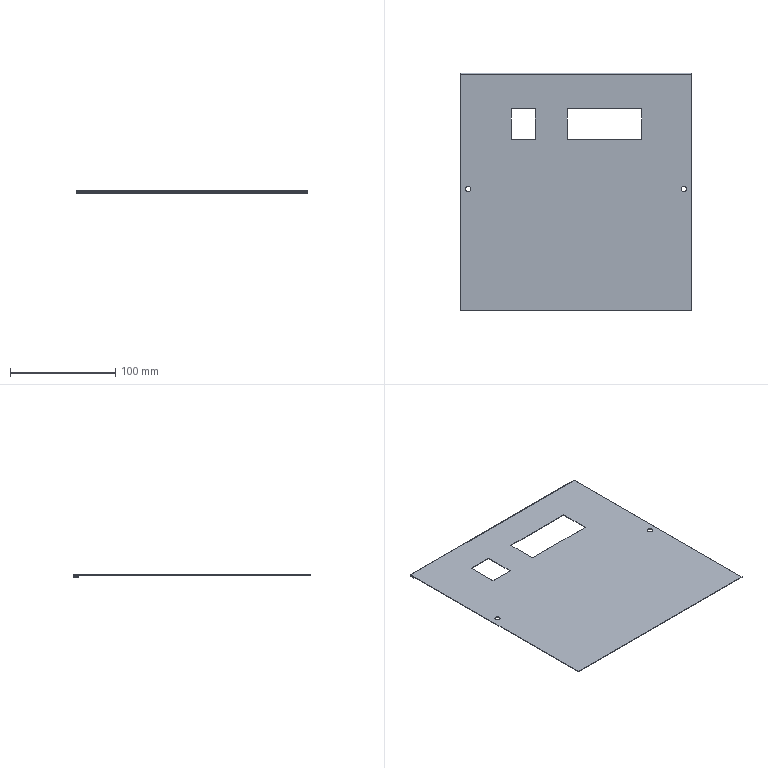Part | SolidWorks | features 3DProfileFeature 1, FlatPattern 1, Hem 1, HoleWzd 1, ICE 1, SMBaseFlange 1, SheetMetal 1 | 1 solid | 26 faces | box 220 x 226 x 2 mm | volume 24067 mm3 | plane 20 | cylinder 6 | commonest cylinder face diameters 5 x4 1 x1 2 x1
STEP:
#1=CARTESIAN_POINT('',(10.,116.,0.));
#2=VERTEX_POINT('',#1);
#3=CARTESIAN_POINT('',(5.,116.,0.));
#4=VERTEX_POINT('',#3);
#5=CARTESIAN_POINT('',(7.5,116.,0.));
#6=DIRECTION('',(0.,0.,-1.));
#7=DIRECTION('',(-1.,0.,0.));
#8=AXIS2_PLACEMENT_3D('',#5,#6,#7);
#9=CIRCLE('',#8,2.5);
#10=EDGE_CURVE('',#2,#4,#9,.T.);
#11=ORIENTED_EDGE('',*,*,#10,.T.);
#12=CARTESIAN_POINT('',(5.,116.,0.5));
#13=VERTEX_POINT('',#12);
#14=CARTESIAN_POINT('',(5.,116.,0.5));
#15=DIRECTION('',(0.,0.,1.));
#16=VECTOR('',#15,1000.);
#17=LINE('',#14,#16);
#18=EDGE_CURVE('',#4,#13,#17,.T.);
#19=ORIENTED_EDGE('',*,*,#18,.T.);
#20=CARTESIAN_POINT('',(10.,116.,0.5));
#21=VERTEX_POINT('',#20);
#22=CARTESIAN_POINT('',(7.5,116.,0.5));
#23=DIRECTION('',(0.,0.,1.));
#24=DIRECTION('',(1.,0.,0.));
#25=AXIS2_PLACEMENT_3D('',#22,#23,#24);
#26=CIRCLE('',#25,2.5);
#27=EDGE_CURVE('',#13,#21,#26,.T.);
#28=ORIENTED_EDGE('',*,*,#27,.T.);
#29=CARTESIAN_POINT('',(10.,116.,0.5));
#30=DIRECTION('',(0.,0.,1.));
#31=VECTOR('',#30,1000.);
#32=LINE('',#29,#31);
#33=EDGE_CURVE('',#2,#21,#32,.T.);
#34=ORIENTED_EDGE('',*,*,#33,.F.);
#35=EDGE_LOOP('',(#11,#19,#28,#34));
#36=FACE_OUTER_BOUND('',#35,.T.);
#37=CARTESIAN_POINT('',(7.5,116.,0.5));
#38=DIRECTION('',(0.,0.,1.));
#39=DIRECTION('',(1.,0.,0.));
#40=AXIS2_PLACEMENT_3D('',#37,#38,#39);
#41=CYLINDRICAL_SURFACE('',#40,2.5);
#42=ADVANCED_FACE('',(#36),#41,.F.);
#43=CARTESIAN_POINT('',(215.,116.,0.));
#44=VERTEX_POINT('',#43);
#45=CARTESIAN_POINT('',(210.,116.,0.));
#46=VERTEX_POINT('',#45);
#47=CARTESIAN_POINT('',(212.5,116.,0.));
#48=DIRECTION('',(0.,0.,-1.));
#49=DIRECTION('',(-1.,0.,0.));
#50=AXIS2_PLACEMENT_3D('',#47,#48,#49);
#51=CIRCLE('',#50,2.5);
#52=EDGE_CURVE('',#44,#46,#51,.T.);
#53=ORIENTED_EDGE('',*,*,#52,.T.);
#54=CARTESIAN_POINT('',(210.,116.,0.5));
#55=VERTEX_POINT('',#54);
#56=CARTESIAN_POINT('',(210.,116.,0.5));
#57=DIRECTION('',(0.,0.,1.));
#58=VECTOR('',#57,1000.);
#59=LINE('',#56,#58);
#60=EDGE_CURVE('',#46,#55,#59,.T.);
#61=ORIENTED_EDGE('',*,*,#60,.T.);
#62=CARTESIAN_POINT('',(215.,116.,0.5));
#63=VERTEX_POINT('',#62);
#64=CARTESIAN_POINT('',(212.5,116.,0.5));
#65=DIRECTION('',(0.,0.,1.));
#66=DIRECTION('',(1.,0.,0.));
#67=AXIS2_PLACEMENT_3D('',#64,#65,#66);
#68=CIRCLE('',#67,2.5);
#69=EDGE_CURVE('',#55,#63,#68,.T.);
#70=ORIENTED_EDGE('',*,*,#69,.T.);
#71=CARTESIAN_POINT('',(215.,116.,0.5));
#72=DIRECTION('',(0.,0.,1.));
#73=VECTOR('',#72,1000.);
#74=LINE('',#71,#73);
#75=EDGE_CURVE('',#44,#63,#74,.T.);
#76=ORIENTED_EDGE('',*,*,#75,.F.);
#77=EDGE_LOOP('',(#53,#61,#70,#76));
#78=FACE_OUTER_BOUND('',#77,.T.);
#79=CARTESIAN_POINT('',(212.5,116.,0.5));
#80=DIRECTION('',(0.,0.,1.));
#81=DIRECTION('',(1.,0.,0.));
#82=AXIS2_PLACEMENT_3D('',#79,#80,#81);
#83=CYLINDRICAL_SURFACE('',#82,2.5);
#84=ADVANCED_FACE('',(#78),#83,.F.);
#85=CARTESIAN_POINT('',(0.,225.,0.5));
#86=VERTEX_POINT('',#85);
#87=CARTESIAN_POINT('',(0.,0.,0.5));
#88=VERTEX_POINT('',#87);
#89=CARTESIAN_POINT('',(0.,0.,0.5));
#90=DIRECTION('',(0.,-1.,0.));
#91=VECTOR('',#90,1000.);
#92=LINE('',#89,#91);
#93=EDGE_CURVE('',#86,#88,#92,.T.);
#94=ORIENTED_EDGE('',*,*,#93,.F.);
#95=CARTESIAN_POINT('',(0.,225.,0.));
#96=VERTEX_POINT('',#95);
#97=CARTESIAN_POINT('',(0.,225.,0.));
#98=DIRECTION('',(0.,0.,1.));
#99=VECTOR('',#98,1000.);
#100=LINE('',#97,#99);
#101=EDGE_CURVE('',#96,#86,#100,.T.);
#102=ORIENTED_EDGE('',*,*,#101,.F.);
#103=CARTESIAN_POINT('',(0.,0.,0.));
#104=VERTEX_POINT('',#103);
#105=CARTESIAN_POINT('',(0.,0.,0.));
#106=DIRECTION('',(0.,-1.,0.));
#107=VECTOR('',#106,1000.);
#108=LINE('',#105,#107);
#109=EDGE_CURVE('',#96,#104,#108,.T.);
#110=ORIENTED_EDGE('',*,*,#109,.T.);
#111=CARTESIAN_POINT('',(0.,0.,0.5));
#112=DIRECTION('',(0.,0.,-1.));
#113=VECTOR('',#112,1000.);
#114=LINE('',#111,#113);
#115=EDGE_CURVE('',#88,#104,#114,.T.);
#116=ORIENTED_EDGE('',*,*,#115,.F.);
#117=EDGE_LOOP('',(#94,#102,#110,#116));
#118=FACE_OUTER_BOUND('',#117,.T.);
#119=CARTESIAN_POINT('',(0.,0.,0.5));
#120=DIRECTION('',(1.,0.,0.));
#121=DIRECTION('',(0.,0.,-1.));
#122=AXIS2_PLACEMENT_3D('',#119,#120,#121);
#123=PLANE('',#122);
#124=ADVANCED_FACE('',(#118),#123,.F.);
#125=CARTESIAN_POINT('',(220.,0.,0.));
#126=VERTEX_POINT('',#125);
#127=CARTESIAN_POINT('',(0.,0.,0.));
#128=DIRECTION('',(1.,0.,0.));
#129=VECTOR('',#128,1000.);
#130=LINE('',#127,#129);
#131=EDGE_CURVE('',#104,#126,#130,.T.);
#132=ORIENTED_EDGE('',*,*,#131,.T.);
#133=CARTESIAN_POINT('',(220.,0.,0.5));
#134=VERTEX_POINT('',#133);
#135=CARTESIAN_POINT('',(220.,0.,0.5));
#136=DIRECTION('',(0.,0.,-1.));
#137=VECTOR('',#136,1000.);
#138=LINE('',#135,#137);
#139=EDGE_CURVE('',#134,#126,#138,.T.);
#140=ORIENTED_EDGE('',*,*,#139,.F.);
#141=CARTESIAN_POINT('',(0.,0.,0.5));
#142=DIRECTION('',(1.,0.,0.));
#143=VECTOR('',#142,1000.);
#144=LINE('',#141,#143);
#145=EDGE_CURVE('',#88,#134,#144,.T.);
#146=ORIENTED_EDGE('',*,*,#145,.F.);
#147=ORIENTED_EDGE('',*,*,#115,.T.);
#148=EDGE_LOOP('',(#132,#140,#146,#147));
#149=FACE_OUTER_BOUND('',#148,.T.);
#150=CARTESIAN_POINT('',(0.,0.,0.5));
#151=DIRECTION('',(0.,1.,0.));
#152=DIRECTION('',(0.,0.,1.));
#153=AXIS2_PLACEMENT_3D('',#150,#151,#152);
#154=PLANE('',#153);
#155=ADVANCED_FACE('',(#149),#154,.F.);
#156=CARTESIAN_POINT('',(220.,225.,0.));
#157=VERTEX_POINT('',#156);
#158=CARTESIAN_POINT('',(220.,0.,0.));
#159=DIRECTION('',(0.,1.,0.));
#160=VECTOR('',#159,1000.);
#161=LINE('',#158,#160);
#162=EDGE_CURVE('',#126,#157,#161,.T.);
#163=ORIENTED_EDGE('',*,*,#162,.T.);
#164=CARTESIAN_POINT('',(220.,225.,0.5));
#165=VERTEX_POINT('',#164);
#166=CARTESIAN_POINT('',(220.,225.,0.));
#167=DIRECTION('',(0.,0.,1.));
#168=VECTOR('',#167,1000.);
#169=LINE('',#166,#168);
#170=EDGE_CURVE('',#157,#165,#169,.T.);
#171=ORIENTED_EDGE('',*,*,#170,.T.);
#172=CARTESIAN_POINT('',(220.,0.,0.5));
#173=DIRECTION('',(0.,1.,0.));
#174=VECTOR('',#173,1000.);
#175=LINE('',#172,#174);
#176=EDGE_CURVE('',#134,#165,#175,.T.);
#177=ORIENTED_EDGE('',*,*,#176,.F.);
#178=ORIENTED_EDGE('',*,*,#139,.T.);
#179=EDGE_LOOP('',(#163,#171,#177,#178));
#180=FACE_OUTER_BOUND('',#179,.T.);
#181=CARTESIAN_POINT('',(220.,0.,0.5));
#182=DIRECTION('',(-1.,0.,0.));
#183=DIRECTION('',(0.,0.,1.));
#184=AXIS2_PLACEMENT_3D('',#181,#182,#183);
#185=PLANE('',#184);
#186=ADVANCED_FACE('',(#180),#185,.F.);
#187=CARTESIAN_POINT('',(7.5,116.,0.5));
#188=DIRECTION('',(0.,0.,1.));
#189=DIRECTION('',(1.,0.,0.));
#190=AXIS2_PLACEMENT_3D('',#187,#188,#189);
#191=CIRCLE('',#190,2.5);
#192=EDGE_CURVE('',#21,#13,#191,.T.);
#193=ORIENTED_EDGE('',*,*,#192,.F.);
#194=ORIENTED_EDGE('',*,*,#27,.F.);
#195=EDGE_LOOP('',(#193,#194));
#196=FACE_BOUND('',#195,.T.);
#197=CARTESIAN_POINT('',(212.5,116.,0.5));
#198=DIRECTION('',(0.,0.,1.));
#199=DIRECTION('',(1.,0.,0.));
#200=AXIS2_PLACEMENT_3D('',#197,#198,#199);
#201=CIRCLE('',#200,2.5);
#202=EDGE_CURVE('',#63,#55,#201,.T.);
#203=ORIENTED_EDGE('',*,*,#202,.F.);
#204=ORIENTED_EDGE('',*,*,#69,.F.);
#205=EDGE_LOOP('',(#203,#204));
#206=FACE_BOUND('',#205,.T.);
#207=CARTESIAN_POINT('',(101.5,163.,0.5));
#208=VERTEX_POINT('',#207);
#209=CARTESIAN_POINT('',(172.5,163.,0.5));
#210=VERTEX_POINT('',#209);
#211=CARTESIAN_POINT('',(101.5,163.,0.5));
#212=DIRECTION('',(1.,0.,0.));
#213=VECTOR('',#212,1000.);
#214=LINE('',#211,#213);
#215=EDGE_CURVE('',#208,#210,#214,.T.);
#216=ORIENTED_EDGE('',*,*,#215,.F.);
#217=CARTESIAN_POINT('',(101.5,192.,0.5));
#218=VERTEX_POINT('',#217);
#219=CARTESIAN_POINT('',(101.5,192.,0.5));
#220=DIRECTION('',(0.,-1.,0.));
#221=VECTOR('',#220,1000.);
#222=LINE('',#219,#221);
#223=EDGE_CURVE('',#218,#208,#222,.T.);
#224=ORIENTED_EDGE('',*,*,#223,.F.);
#225=CARTESIAN_POINT('',(172.5,192.,0.5));
#226=VERTEX_POINT('',#225);
#227=CARTESIAN_POINT('',(101.5,192.,0.5));
#228=DIRECTION('',(-1.,0.,0.));
#229=VECTOR('',#228,1000.);
#230=LINE('',#227,#229);
#231=EDGE_CURVE('',#226,#218,#230,.T.);
#232=ORIENTED_EDGE('',*,*,#231,.F.);
#233=CARTESIAN_POINT('',(172.5,192.,0.5));
#234=DIRECTION('',(0.,1.,0.));
#235=VECTOR('',#234,1000.);
#236=LINE('',#233,#235);
#237=EDGE_CURVE('',#210,#226,#236,.T.);
#238=ORIENTED_EDGE('',*,*,#237,.F.);
#239=EDGE_LOOP('',(#216,#224,#232,#238));
#240=FACE_BOUND('',#239,.T.);
#241=CARTESIAN_POINT('',(48.5,163.,0.5));
#242=VERTEX_POINT('',#241);
#243=CARTESIAN_POINT('',(71.5,163.,0.5));
#244=VERTEX_POINT('',#243);
#245=CARTESIAN_POINT('',(48.5,163.,0.5));
#246=DIRECTION('',(1.,0.,0.));
#247=VECTOR('',#246,1000.);
#248=LINE('',#245,#247);
#249=EDGE_CURVE('',#242,#244,#248,.T.);
#250=ORIENTED_EDGE('',*,*,#249,.F.);
#251=CARTESIAN_POINT('',(48.5,192.,0.5));
#252=VERTEX_POINT('',#251);
#253=CARTESIAN_POINT('',(48.5,192.,0.5));
#254=DIRECTION('',(0.,-1.,0.));
#255=VECTOR('',#254,1000.);
#256=LINE('',#253,#255);
#257=EDGE_CURVE('',#252,#242,#256,.T.);
#258=ORIENTED_EDGE('',*,*,#257,.F.);
#259=CARTESIAN_POINT('',(71.5,192.,0.5));
#260=VERTEX_POINT('',#259);
#261=CARTESIAN_POINT('',(48.5,192.,0.5));
#262=DIRECTION('',(-1.,0.,0.));
#263=VECTOR('',#262,1000.);
#264=LINE('',#261,#263);
#265=EDGE_CURVE('',#260,#252,#264,.T.);
#266=ORIENTED_EDGE('',*,*,#265,.F.);
#267=CARTESIAN_POINT('',(71.5,192.,0.5));
#268=DIRECTION('',(0.,1.,0.));
#269=VECTOR('',#268,1000.);
#270=LINE('',#267,#269);
#271=EDGE_CURVE('',#244,#260,#270,.T.);
#272=ORIENTED_EDGE('',*,*,#271,.F.);
#273=EDGE_LOOP('',(#250,#258,#266,#272));
#274=FACE_BOUND('',#273,.T.);
#275=ORIENTED_EDGE('',*,*,#176,.T.);
#276=CARTESIAN_POINT('',(220.,225.,0.5));
#277=DIRECTION('',(-1.,0.,0.));
#278=VECTOR('',#277,1000.);
#279=LINE('',#276,#278);
#280=EDGE_CURVE('',#165,#86,#279,.T.);
#281=ORIENTED_EDGE('',*,*,#280,.T.);
#282=ORIENTED_EDGE('',*,*,#93,.T.);
#283=ORIENTED_EDGE('',*,*,#145,.T.);
#284=EDGE_LOOP('',(#275,#281,#282,#283));
#285=FACE_OUTER_BOUND('',#284,.T.);
#286=CARTESIAN_POINT('',(0.,226.,0.5));
#287=DIRECTION('',(0.,0.,-1.));
#288=DIRECTION('',(-1.,0.,0.));
#289=AXIS2_PLACEMENT_3D('',#286,#287,#288);
#290=PLANE('',#289);
#291=ADVANCED_FACE('',(#196,#206,#240,#274,#285),#290,.F.);
#292=ORIENTED_EDGE('',*,*,#10,.F.);
#293=CARTESIAN_POINT('',(7.5,116.,0.));
#294=DIRECTION('',(0.,0.,-1.));
#295=DIRECTION('',(-1.,0.,0.));
#296=AXIS2_PLACEMENT_3D('',#293,#294,#295);
#297=CIRCLE('',#296,2.5);
#298=EDGE_CURVE('',#4,#2,#297,.T.);
#299=ORIENTED_EDGE('',*,*,#298,.F.);
#300=EDGE_LOOP('',(#292,#299));
#301=FACE_BOUND('',#300,.T.);
#302=ORIENTED_EDGE('',*,*,#52,.F.);
#303=CARTESIAN_POINT('',(212.5,116.,0.));
#304=DIRECTION('',(0.,0.,-1.));
#305=DIRECTION('',(-1.,0.,0.));
#306=AXIS2_PLACEMENT_3D('',#303,#304,#305);
#307=CIRCLE('',#306,2.5);
#308=EDGE_CURVE('',#46,#44,#307,.T.);
#309=ORIENTED_EDGE('',*,*,#308,.F.);
#310=EDGE_LOOP('',(#302,#309));
#311=FACE_BOUND('',#310,.T.);
#312=CARTESIAN_POINT('',(101.5,163.,0.));
#313=VERTEX_POINT('',#312);
#314=CARTESIAN_POINT('',(101.5,192.,0.));
#315=VERTEX_POINT('',#314);
#316=CARTESIAN_POINT('',(101.5,226.,0.));
#317=DIRECTION('',(0.,1.,0.));
#318=VECTOR('',#317,1000.);
#319=LINE('',#316,#318);
#320=EDGE_CURVE('',#313,#315,#319,.T.);
#321=ORIENTED_EDGE('',*,*,#320,.F.);
#322=CARTESIAN_POINT('',(172.5,163.,0.));
#323=VERTEX_POINT('',#322);
#324=CARTESIAN_POINT('',(0.,163.,0.));
#325=DIRECTION('',(-1.,0.,0.));
#326=VECTOR('',#325,1000.);
#327=LINE('',#324,#326);
#328=EDGE_CURVE('',#323,#313,#327,.T.);
#329=ORIENTED_EDGE('',*,*,#328,.F.);
#330=CARTESIAN_POINT('',(172.5,192.,0.));
#331=VERTEX_POINT('',#330);
#332=CARTESIAN_POINT('',(172.5,226.,0.));
#333=DIRECTION('',(0.,-1.,0.));
#334=VECTOR('',#333,1000.);
#335=LINE('',#332,#334);
#336=EDGE_CURVE('',#331,#323,#335,.T.);
#337=ORIENTED_EDGE('',*,*,#336,.F.);
#338=CARTESIAN_POINT('',(0.,192.,0.));
#339=DIRECTION('',(1.,0.,0.));
#340=VECTOR('',#339,1000.);
#341=LINE('',#338,#340);
#342=EDGE_CURVE('',#315,#331,#341,.T.);
#343=ORIENTED_EDGE('',*,*,#342,.F.);
#344=EDGE_LOOP('',(#321,#329,#337,#343));
#345=FACE_BOUND('',#344,.T.);
#346=CARTESIAN_POINT('',(48.5,163.,0.));
#347=VERTEX_POINT('',#346);
#348=CARTESIAN_POINT('',(48.5,192.,0.));
#349=VERTEX_POINT('',#348);
#350=CARTESIAN_POINT('',(48.5,226.,0.));
#351=DIRECTION('',(0.,1.,0.));
#352=VECTOR('',#351,1000.);
#353=LINE('',#350,#352);
#354=EDGE_CURVE('',#347,#349,#353,.T.);
#355=ORIENTED_EDGE('',*,*,#354,.F.);
#356=CARTESIAN_POINT('',(71.5,163.,0.));
#357=VERTEX_POINT('',#356);
#358=CARTESIAN_POINT('',(0.,163.,0.));
#359=DIRECTION('',(-1.,0.,0.));
#360=VECTOR('',#359,1000.);
#361=LINE('',#358,#360);
#362=EDGE_CURVE('',#357,#347,#361,.T.);
#363=ORIENTED_EDGE('',*,*,#362,.F.);
#364=CARTESIAN_POINT('',(71.5,192.,0.));
#365=VERTEX_POINT('',#364);
#366=CARTESIAN_POINT('',(71.5,226.,0.));
#367=DIRECTION('',(0.,-1.,0.));
#368=VECTOR('',#367,1000.);
#369=LINE('',#366,#368);
#370=EDGE_CURVE('',#365,#357,#369,.T.);
#371=ORIENTED_EDGE('',*,*,#370,.F.);
#372=CARTESIAN_POINT('',(0.,192.,0.));
#373=DIRECTION('',(1.,0.,0.));
#374=VECTOR('',#373,1000.);
#375=LINE('',#372,#374);
#376=EDGE_CURVE('',#349,#365,#375,.T.);
#377=ORIENTED_EDGE('',*,*,#376,.F.);
#378=EDGE_LOOP('',(#355,#363,#371,#377));
#379=FACE_BOUND('',#378,.T.);
#380=CARTESIAN_POINT('',(220.,225.,0.));
#381=DIRECTION('',(-1.,0.,0.));
#382=VECTOR('',#381,1000.);
#383=LINE('',#380,#382);
#384=EDGE_CURVE('',#157,#96,#383,.T.);
#385=ORIENTED_EDGE('',*,*,#384,.F.);
#386=ORIENTED_EDGE('',*,*,#162,.F.);
#387=ORIENTED_EDGE('',*,*,#131,.F.);
#388=ORIENTED_EDGE('',*,*,#109,.F.);
#389=EDGE_LOOP('',(#385,#386,#387,#388));
#390=FACE_OUTER_BOUND('',#389,.T.);
#391=CARTESIAN_POINT('',(0.,226.,0.));
#392=DIRECTION('',(0.,0.,-1.));
#393=DIRECTION('',(-1.,0.,0.));
#394=AXIS2_PLACEMENT_3D('',#391,#392,#393);
#395=PLANE('',#394);
#396=ADVANCED_FACE('',(#301,#311,#345,#379,#390),#395,.T.);
#397=CARTESIAN_POINT('',(220.,225.,-1.));
#398=VERTEX_POINT('',#397);
#399=CARTESIAN_POINT('',(220.,225.,-1.5));
#400=VERTEX_POINT('',#399);
#401=CARTESIAN_POINT('',(220.,225.,-1.5));
#402=DIRECTION('',(0.,0.,-1.));
#403=VECTOR('',#402,1000.);
#404=LINE('',#401,#403);
#405=EDGE_CURVE('',#398,#400,#404,.T.);
#406=ORIENTED_EDGE('',*,*,#405,.F.);
#407=CARTESIAN_POINT('',(220.,221.,-1.));
#408=VERTEX_POINT('',#407);
#409=CARTESIAN_POINT('',(220.,223.,-1.));
#410=DIRECTION('',(0.,1.,0.));
#411=VECTOR('',#410,1000.);
#412=LINE('',#409,#411);
#413=EDGE_CURVE('',#408,#398,#412,.T.);
#414=ORIENTED_EDGE('',*,*,#413,.F.);
#415=CARTESIAN_POINT('',(220.,221.,-1.5));
#416=VERTEX_POINT('',#415);
#417=CARTESIAN_POINT('',(220.,221.,-1.5));
#418=DIRECTION('',(0.,0.,-1.));
#419=VECTOR('',#418,1000.);
#420=LINE('',#417,#419);
#421=EDGE_CURVE('',#408,#416,#420,.T.);
#422=ORIENTED_EDGE('',*,*,#421,.T.);
#423=CARTESIAN_POINT('',(220.,223.,-1.5));
#424=DIRECTION('',(0.,1.,0.));
#425=VECTOR('',#424,1000.);
#426=LINE('',#423,#425);
#427=EDGE_CURVE('',#416,#400,#426,.T.);
#428=ORIENTED_EDGE('',*,*,#427,.T.);
#429=EDGE_LOOP('',(#406,#414,#422,#428));
#430=FACE_OUTER_BOUND('',#429,.T.);
#431=CARTESIAN_POINT('',(220.,223.,-1.5));
#432=DIRECTION('',(-1.,0.,0.));
#433=DIRECTION('',(0.,1.,0.));
#434=AXIS2_PLACEMENT_3D('',#431,#432,#433);
#435=PLANE('',#434);
#436=ADVANCED_FACE('',(#430),#435,.F.);
#437=ORIENTED_EDGE('',*,*,#421,.F.);
#438=CARTESIAN_POINT('',(0.,221.,-1.));
#439=VERTEX_POINT('',#438);
#440=CARTESIAN_POINT('',(110.,221.,-1.));
#441=DIRECTION('',(1.,0.,0.));
#442=VECTOR('',#441,1000.);
#443=LINE('',#440,#442);
#444=EDGE_CURVE('',#439,#408,#443,.T.);
#445=ORIENTED_EDGE('',*,*,#444,.F.);
#446=CARTESIAN_POINT('',(0.,221.,-1.5));
#447=VERTEX_POINT('',#446);
#448=CARTESIAN_POINT('',(0.,221.,-1.5));
#449=DIRECTION('',(0.,0.,-1.));
#450=VECTOR('',#449,1000.);
#451=LINE('',#448,#450);
#452=EDGE_CURVE('',#439,#447,#451,.T.);
#453=ORIENTED_EDGE('',*,*,#452,.T.);
#454=CARTESIAN_POINT('',(110.,221.,-1.5));
#455=DIRECTION('',(1.,0.,0.));
#456=VECTOR('',#455,1000.);
#457=LINE('',#454,#456);
#458=EDGE_CURVE('',#447,#416,#457,.T.);
#459=ORIENTED_EDGE('',*,*,#458,.T.);
#460=EDGE_LOOP('',(#437,#445,#453,#459));
#461=FACE_OUTER_BOUND('',#460,.T.);
#462=CARTESIAN_POINT('',(110.,221.,-1.5));
#463=DIRECTION('',(0.,1.,0.));
#464=DIRECTION('',(1.,0.,0.));
#465=AXIS2_PLACEMENT_3D('',#462,#463,#464);
#466=PLANE('',#465);
#467=ADVANCED_FACE('',(#461),#466,.F.);
#468=ORIENTED_EDGE('',*,*,#458,.F.);
#469=CARTESIAN_POINT('',(0.,225.,-1.5));
#470=VERTEX_POINT('',#469);
#471=CARTESIAN_POINT('',(0.,223.,-1.5));
#472=DIRECTION('',(0.,-1.,0.));
#473=VECTOR('',#472,1000.);
#474=LINE('',#471,#473);
#475=EDGE_CURVE('',#470,#447,#474,.T.);
#476=ORIENTED_EDGE('',*,*,#475,.F.);
#477=CARTESIAN_POINT('',(110.,225.,-1.5));
#478=DIRECTION('',(-1.,0.,0.));
#479=VECTOR('',#478,1000.);
#480=LINE('',#477,#479);
#481=EDGE_CURVE('',#400,#470,#480,.T.);
#482=ORIENTED_EDGE('',*,*,#481,.F.);
#483=ORIENTED_EDGE('',*,*,#427,.F.);
#484=EDGE_LOOP('',(#468,#476,#482,#483));
#485=FACE_OUTER_BOUND('',#484,.T.);
#486=CARTESIAN_POINT('',(110.,223.,-1.5));
#487=DIRECTION('',(0.,0.,-1.));
#488=DIRECTION('',(-1.,0.,0.));
#489=AXIS2_PLACEMENT_3D('',#486,#487,#488);
#490=PLANE('',#489);
#491=ADVANCED_FACE('',(#485),#490,.T.);
#492=CARTESIAN_POINT('',(0.,225.,-1.));
#493=VERTEX_POINT('',#492);
#494=CARTESIAN_POINT('',(0.,223.,-1.));
#495=DIRECTION('',(0.,-1.,0.));
#496=VECTOR('',#495,1000.);
#497=LINE('',#494,#496);
#498=EDGE_CURVE('',#493,#439,#497,.T.);
#499=ORIENTED_EDGE('',*,*,#498,.F.);
#500=CARTESIAN_POINT('',(0.,225.,-1.5));
#501=DIRECTION('',(0.,0.,-1.));
#502=VECTOR('',#501,1000.);
#503=LINE('',#500,#502);
#504=EDGE_CURVE('',#493,#470,#503,.T.);
#505=ORIENTED_EDGE('',*,*,#504,.T.);
#506=ORIENTED_EDGE('',*,*,#475,.T.);
#507=ORIENTED_EDGE('',*,*,#452,.F.);
#508=EDGE_LOOP('',(#499,#505,#506,#507));
#509=FACE_OUTER_BOUND('',#508,.T.);
#510=CARTESIAN_POINT('',(0.,223.,-1.5));
#511=DIRECTION('',(1.,0.,0.));
#512=DIRECTION('',(0.,-1.,0.));
#513=AXIS2_PLACEMENT_3D('',#510,#511,#512);
#514=PLANE('',#513);
#515=ADVANCED_FACE('',(#509),#514,.F.);
#516=ORIENTED_EDGE('',*,*,#444,.T.);
#517=ORIENTED_EDGE('',*,*,#413,.T.);
#518=CARTESIAN_POINT('',(110.,225.,-1.));
#519=DIRECTION('',(-1.,0.,0.));
#520=VECTOR('',#519,1000.);
#521=LINE('',#518,#520);
#522=EDGE_CURVE('',#398,#493,#521,.T.);
#523=ORIENTED_EDGE('',*,*,#522,.T.);
#524=ORIENTED_EDGE('',*,*,#498,.T.);
#525=EDGE_LOOP('',(#516,#517,#523,#524));
#526=FACE_OUTER_BOUND('',#525,.T.);
#527=CARTESIAN_POINT('',(110.,223.,-1.));
#528=DIRECTION('',(0.,0.,-1.));
#529=DIRECTION('',(-1.,0.,0.));
#530=AXIS2_PLACEMENT_3D('',#527,#528,#529);
#531=PLANE('',#530);
#532=ADVANCED_FACE('',(#526),#531,.F.);
#533=ORIENTED_EDGE('',*,*,#504,.F.);
#534=CARTESIAN_POINT('',(0.,225.,-0.5));
#535=DIRECTION('',(-1.,0.,0.));
#536=DIRECTION('',(0.,0.,-1.));
#537=AXIS2_PLACEMENT_3D('',#534,#535,#536);
#538=CIRCLE('',#537,0.5);
#539=EDGE_CURVE('',#96,#493,#538,.T.);
#540=ORIENTED_EDGE('',*,*,#539,.F.);
#541=ORIENTED_EDGE('',*,*,#101,.T.);
#542=CARTESIAN_POINT('',(0.,225.,-0.5));
#543=DIRECTION('',(-1.,0.,0.));
#544=DIRECTION('',(0.,0.,-1.));
#545=AXIS2_PLACEMENT_3D('',#542,#543,#544);
#546=CIRCLE('',#545,1.);
#547=EDGE_CURVE('',#86,#470,#546,.T.);
#548=ORIENTED_EDGE('',*,*,#547,.T.);
#549=EDGE_LOOP('',(#533,#540,#541,#548));
#550=FACE_OUTER_BOUND('',#549,.T.);
#551=CARTESIAN_POINT('',(0.,225.,-0.5));
#552=DIRECTION('',(-1.,0.,0.));
#553=DIRECTION('',(0.,0.,1.));
#554=AXIS2_PLACEMENT_3D('',#551,#552,#553);
#555=PLANE('',#554);
#556=ADVANCED_FACE('',(#550),#555,.T.);
#557=ORIENTED_EDGE('',*,*,#280,.F.);
#558=CARTESIAN_POINT('',(220.,225.,-0.5));
#559=DIRECTION('',(1.,0.,0.));
#560=DIRECTION('',(0.,0.,-1.));
#561=AXIS2_PLACEMENT_3D('',#558,#559,#560);
#562=CIRCLE('',#561,1.);
#563=EDGE_CURVE('',#400,#165,#562,.T.);
#564=ORIENTED_EDGE('',*,*,#563,.F.);
#565=ORIENTED_EDGE('',*,*,#481,.T.);
#566=ORIENTED_EDGE('',*,*,#547,.F.);
#567=EDGE_LOOP('',(#557,#564,#565,#566));
#568=FACE_OUTER_BOUND('',#567,.T.);
#569=CARTESIAN_POINT('',(220.,225.,-0.5));
#570=DIRECTION('',(1.,0.,0.));
#571=DIRECTION('',(0.,0.,-1.));
#572=AXIS2_PLACEMENT_3D('',#569,#570,#571);
#573=CYLINDRICAL_SURFACE('',#572,1.);
#574=ADVANCED_FACE('',(#568),#573,.T.);
#575=CARTESIAN_POINT('',(220.,225.,-0.5));
#576=DIRECTION('',(1.,0.,0.));
#577=DIRECTION('',(0.,0.,-1.));
#578=AXIS2_PLACEMENT_3D('',#575,#576,#577);
#579=CIRCLE('',#578,0.5);
#580=EDGE_CURVE('',#398,#157,#579,.T.);
#581=ORIENTED_EDGE('',*,*,#580,.F.);
#582=ORIENTED_EDGE('',*,*,#405,.T.);
#583=ORIENTED_EDGE('',*,*,#563,.T.);
#584=ORIENTED_EDGE('',*,*,#170,.F.);
#585=EDGE_LOOP('',(#581,#582,#583,#584));
#586=FACE_OUTER_BOUND('',#585,.T.);
#587=CARTESIAN_POINT('',(220.,225.,-0.5));
#588=DIRECTION('',(-1.,0.,0.));
#589=DIRECTION('',(0.,0.,1.));
#590=AXIS2_PLACEMENT_3D('',#587,#588,#589);
#591=PLANE('',#590);
#592=ADVANCED_FACE('',(#586),#591,.F.);
#593=ORIENTED_EDGE('',*,*,#384,.T.);
#594=ORIENTED_EDGE('',*,*,#539,.T.);
#595=ORIENTED_EDGE('',*,*,#522,.F.);
#596=ORIENTED_EDGE('',*,*,#580,.T.);
#597=EDGE_LOOP('',(#593,#594,#595,#596));
#598=FACE_OUTER_BOUND('',#597,.T.);
#599=CARTESIAN_POINT('',(220.,225.,-0.5));
#600=DIRECTION('',(1.,0.,0.));
#601=DIRECTION('',(0.,0.,-1.));
#602=AXIS2_PLACEMENT_3D('',#599,#600,#601);
#603=CYLINDRICAL_SURFACE('',#602,0.5);
#604=ADVANCED_FACE('',(#598),#603,.F.);
#605=ORIENTED_EDGE('',*,*,#354,.T.);
#606=CARTESIAN_POINT('',(48.5,192.,-9.5));
#607=DIRECTION('',(0.,0.,1.));
#608=VECTOR('',#607,1000.);
#609=LINE('',#606,#608);
#610=EDGE_CURVE('',#349,#252,#609,.T.);
#611=ORIENTED_EDGE('',*,*,#610,.T.);
#612=ORIENTED_EDGE('',*,*,#257,.T.);
#613=CARTESIAN_POINT('',(48.5,163.,-9.5));
#614=DIRECTION('',(0.,0.,1.));
#615=VECTOR('',#614,1000.);
#616=LINE('',#613,#615);
#617=EDGE_CURVE('',#347,#242,#616,.T.);
#618=ORIENTED_EDGE('',*,*,#617,.F.);
#619=EDGE_LOOP('',(#605,#611,#612,#618));
#620=FACE_OUTER_BOUND('',#619,.T.);
#621=CARTESIAN_POINT('',(48.5,192.,-9.5));
#622=DIRECTION('',(-1.,0.,0.));
#623=DIRECTION('',(0.,-1.,0.));
#624=AXIS2_PLACEMENT_3D('',#621,#622,#623);
#625=PLANE('',#624);
#626=ADVANCED_FACE('',(#620),#625,.F.);
#627=ORIENTED_EDGE('',*,*,#376,.T.);
#628=CARTESIAN_POINT('',(71.5,192.,-9.5));
#629=DIRECTION('',(0.,0.,1.));
#630=VECTOR('',#629,1000.);
#631=LINE('',#628,#630);
#632=EDGE_CURVE('',#365,#260,#631,.T.);
#633=ORIENTED_EDGE('',*,*,#632,.T.);
#634=ORIENTED_EDGE('',*,*,#265,.T.);
#635=ORIENTED_EDGE('',*,*,#610,.F.);
#636=EDGE_LOOP('',(#627,#633,#634,#635));
#637=FACE_OUTER_BOUND('',#636,.T.);
#638=CARTESIAN_POINT('',(48.5,192.,-9.5));
#639=DIRECTION('',(0.,1.,0.));
#640=DIRECTION('',(0.,0.,1.));
#641=AXIS2_PLACEMENT_3D('',#638,#639,#640);
#642=PLANE('',#641);
#643=ADVANCED_FACE('',(#637),#642,.F.);
#644=ORIENTED_EDGE('',*,*,#370,.T.);
#645=CARTESIAN_POINT('',(71.5,163.,-9.5));
#646=DIRECTION('',(0.,0.,1.));
#647=VECTOR('',#646,1000.);
#648=LINE('',#645,#647);
#649=EDGE_CURVE('',#357,#244,#648,.T.);
#650=ORIENTED_EDGE('',*,*,#649,.T.);
#651=ORIENTED_EDGE('',*,*,#271,.T.);
#652=ORIENTED_EDGE('',*,*,#632,.F.);
#653=EDGE_LOOP('',(#644,#650,#651,#652));
#654=FACE_OUTER_BOUND('',#653,.T.);
#655=CARTESIAN_POINT('',(71.5,192.,-9.5));
#656=DIRECTION('',(1.,0.,0.));
#657=DIRECTION('',(0.,0.,-1.));
#658=AXIS2_PLACEMENT_3D('',#655,#656,#657);
#659=PLANE('',#658);
#660=ADVANCED_FACE('',(#654),#659,.F.);
#661=ORIENTED_EDGE('',*,*,#362,.T.);
#662=ORIENTED_EDGE('',*,*,#617,.T.);
#663=ORIENTED_EDGE('',*,*,#249,.T.);
#664=ORIENTED_EDGE('',*,*,#649,.F.);
#665=EDGE_LOOP('',(#661,#662,#663,#664));
#666=FACE_OUTER_BOUND('',#665,.T.);
#667=CARTESIAN_POINT('',(48.5,163.,-9.5));
#668=DIRECTION('',(0.,-1.,0.));
#669=DIRECTION('',(0.,0.,-1.));
#670=AXIS2_PLACEMENT_3D('',#667,#668,#669);
#671=PLANE('',#670);
#672=ADVANCED_FACE('',(#666),#671,.F.);
#673=ORIENTED_EDGE('',*,*,#320,.T.);
#674=CARTESIAN_POINT('',(101.5,192.,-9.5));
#675=DIRECTION('',(0.,0.,1.));
#676=VECTOR('',#675,1000.);
#677=LINE('',#674,#676);
#678=EDGE_CURVE('',#315,#218,#677,.T.);
#679=ORIENTED_EDGE('',*,*,#678,.T.);
#680=ORIENTED_EDGE('',*,*,#223,.T.);
#681=CARTESIAN_POINT('',(101.5,163.,-9.5));
#682=DIRECTION('',(0.,0.,1.));
#683=VECTOR('',#682,1000.);
#684=LINE('',#681,#683);
#685=EDGE_CURVE('',#313,#208,#684,.T.);
#686=ORIENTED_EDGE('',*,*,#685,.F.);
#687=EDGE_LOOP('',(#673,#679,#680,#686));
#688=FACE_OUTER_BOUND('',#687,.T.);
#689=CARTESIAN_POINT('',(101.5,192.,-9.5));
#690=DIRECTION('',(-1.,0.,0.));
#691=DIRECTION('',(0.,0.,1.));
#692=AXIS2_PLACEMENT_3D('',#689,#690,#691);
#693=PLANE('',#692);
#694=ADVANCED_FACE('',(#688),#693,.F.);
#695=ORIENTED_EDGE('',*,*,#342,.T.);
#696=CARTESIAN_POINT('',(172.5,192.,-9.5));
#697=DIRECTION('',(0.,0.,1.));
#698=VECTOR('',#697,1000.);
#699=LINE('',#696,#698);
#700=EDGE_CURVE('',#331,#226,#699,.T.);
#701=ORIENTED_EDGE('',*,*,#700,.T.);
#702=ORIENTED_EDGE('',*,*,#231,.T.);
#703=ORIENTED_EDGE('',*,*,#678,.F.);
#704=EDGE_LOOP('',(#695,#701,#702,#703));
#705=FACE_OUTER_BOUND('',#704,.T.);
#706=CARTESIAN_POINT('',(101.5,192.,-9.5));
#707=DIRECTION('',(0.,1.,0.));
#708=DIRECTION('',(0.,0.,1.));
#709=AXIS2_PLACEMENT_3D('',#706,#707,#708);
#710=PLANE('',#709);
#711=ADVANCED_FACE('',(#705),#710,.F.);
#712=ORIENTED_EDGE('',*,*,#336,.T.);
#713=CARTESIAN_POINT('',(172.5,163.,-9.5));
#714=DIRECTION('',(0.,0.,1.));
#715=VECTOR('',#714,1000.);
#716=LINE('',#713,#715);
#717=EDGE_CURVE('',#323,#210,#716,.T.);
#718=ORIENTED_EDGE('',*,*,#717,.T.);
#719=ORIENTED_EDGE('',*,*,#237,.T.);
#720=ORIENTED_EDGE('',*,*,#700,.F.);
#721=EDGE_LOOP('',(#712,#718,#719,#720));
#722=FACE_OUTER_BOUND('',#721,.T.);
#723=CARTESIAN_POINT('',(172.5,192.,-9.5));
#724=DIRECTION('',(1.,0.,0.));
#725=DIRECTION('',(0.,0.,-1.));
#726=AXIS2_PLACEMENT_3D('',#723,#724,#725);
#727=PLANE('',#726);
#728=ADVANCED_FACE('',(#722),#727,.F.);
#729=ORIENTED_EDGE('',*,*,#328,.T.);
#730=ORIENTED_EDGE('',*,*,#685,.T.);
#731=ORIENTED_EDGE('',*,*,#215,.T.);
#732=ORIENTED_EDGE('',*,*,#717,.F.);
#733=EDGE_LOOP('',(#729,#730,#731,#732));
#734=FACE_OUTER_BOUND('',#733,.T.);
#735=CARTESIAN_POINT('',(101.5,163.,-9.5));
#736=DIRECTION('',(0.,-1.,0.));
#737=DIRECTION('',(0.,0.,-1.));
#738=AXIS2_PLACEMENT_3D('',#735,#736,#737);
#739=PLANE('',#738);
#740=ADVANCED_FACE('',(#734),#739,.F.);
#741=ORIENTED_EDGE('',*,*,#60,.F.);
#742=ORIENTED_EDGE('',*,*,#308,.T.);
#743=ORIENTED_EDGE('',*,*,#75,.T.);
#744=ORIENTED_EDGE('',*,*,#202,.T.);
#745=EDGE_LOOP('',(#741,#742,#743,#744));
#746=FACE_OUTER_BOUND('',#745,.T.);
#747=CARTESIAN_POINT('',(212.5,116.,0.5));
#748=DIRECTION('',(0.,0.,1.));
#749=DIRECTION('',(1.,0.,0.));
#750=AXIS2_PLACEMENT_3D('',#747,#748,#749);
#751=CYLINDRICAL_SURFACE('',#750,2.5);
#752=ADVANCED_FACE('',(#746),#751,.F.);
#753=ORIENTED_EDGE('',*,*,#18,.F.);
#754=ORIENTED_EDGE('',*,*,#298,.T.);
#755=ORIENTED_EDGE('',*,*,#33,.T.);
#756=ORIENTED_EDGE('',*,*,#192,.T.);
#757=EDGE_LOOP('',(#753,#754,#755,#756));
#758=FACE_OUTER_BOUND('',#757,.T.);
#759=CARTESIAN_POINT('',(7.5,116.,0.5));
#760=DIRECTION('',(0.,0.,1.));
#761=DIRECTION('',(1.,0.,0.));
#762=AXIS2_PLACEMENT_3D('',#759,#760,#761);
#763=CYLINDRICAL_SURFACE('',#762,2.5);
#764=ADVANCED_FACE('',(#758),#763,.F.);
#765=CLOSED_SHELL('',(#42,#84,#124,#155,#186,#291,#396,#436,#467,#491,#515,#532,#556,#574,#592,#604,#626,#643,#660,#672,#694,#711,#728,#740,#752,#764));
#766=MANIFOLD_SOLID_BREP('',#765);
#767=CARTESIAN_POINT('',(0.,0.,0.));
#768=DIRECTION('',(0.,0.,1.));
#769=DIRECTION('',(1.,0.,0.));
#770=AXIS2_PLACEMENT_3D('',#767,#768,#769);
#771=(LENGTH_UNIT()NAMED_UNIT(*)SI_UNIT(.MILLI.,.METRE.));
#772=UNCERTAINTY_MEASURE_WITH_UNIT(LENGTH_MEASURE(0.00001),#771,'','');
#773=(NAMED_UNIT(*)PLANE_ANGLE_UNIT()SI_UNIT($,.RADIAN.));
#774=(NAMED_UNIT(*)SI_UNIT($,.STERADIAN.)SOLID_ANGLE_UNIT());
#775=(GEOMETRIC_REPRESENTATION_CONTEXT(3)GLOBAL_UNCERTAINTY_ASSIGNED_CONTEXT((#772))GLOBAL_UNIT_ASSIGNED_CONTEXT((#771,#773,#774))REPRESENTATION_CONTEXT('',''));
#776=ADVANCED_BREP_SHAPE_REPRESENTATION('',(#766,#770),#775);